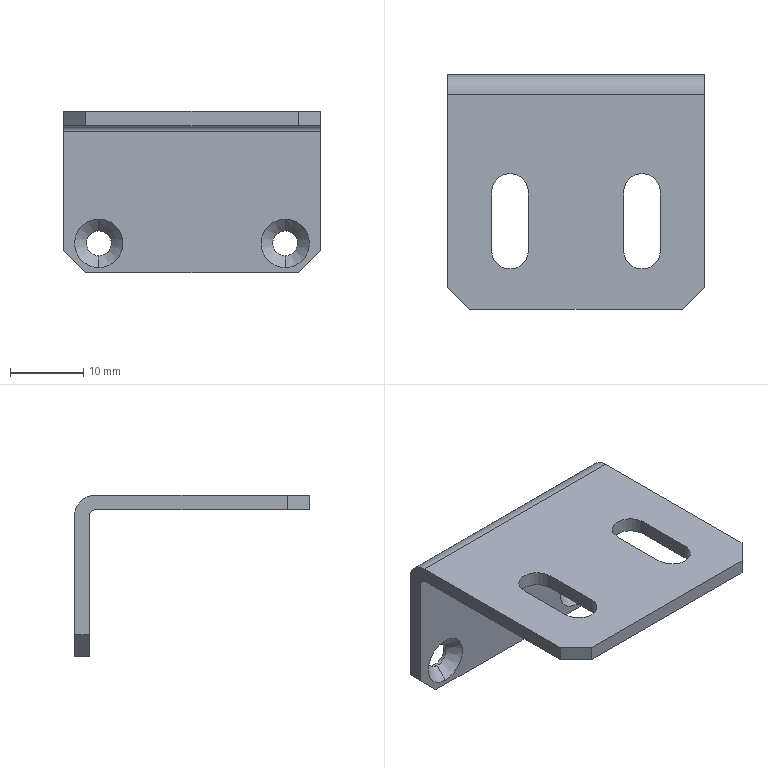Part | STEP file | PN_0018 Sensor bracket | 1 solid | 30 faces | box 35 x 32 x 22 mm | volume 3241 mm3 | plane 16 | cylinder 10 | cone 4 | commonest cylinder face diameters 3.4 x4 5 x4 1.473 x1 5.473 x1